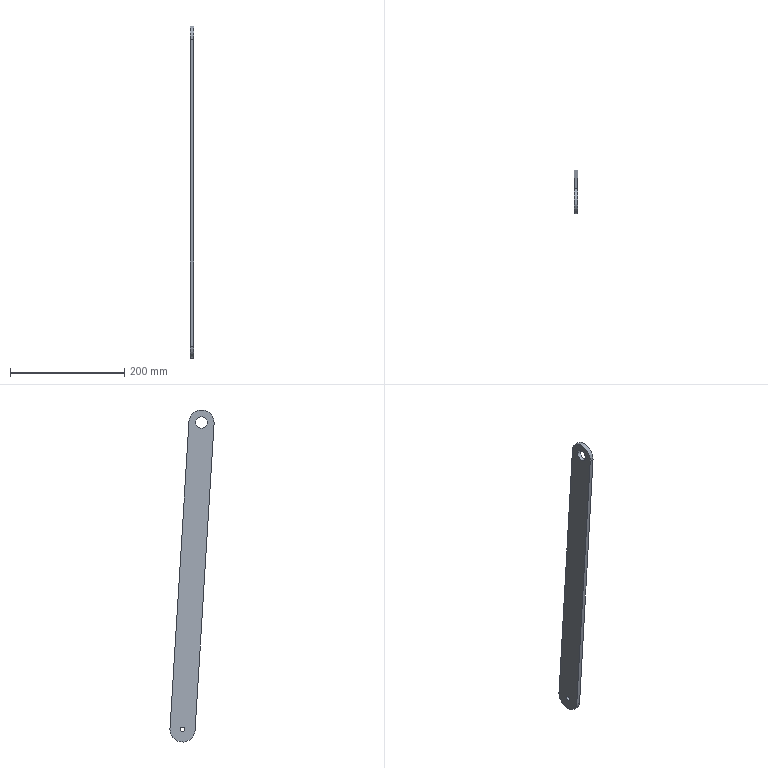Part | SolidWorks | features Extrusion 1 | 1 solid | 11 faces | box 7 x 77.287 x 581.266 mm | volume 173888 mm3 | cylinder 7 | plane 4 | commonest cylinder face diameters 44 x3 8 x2 20 x2
STEP:
#1=CARTESIAN_POINT('',(790.598,-43.287,187.266));
#2=VERTEX_POINT('',#1);
#3=CARTESIAN_POINT('',(790.598,-23.287,187.266));
#4=VERTEX_POINT('',#3);
#5=CARTESIAN_POINT('',(790.598,-33.287,187.266));
#6=DIRECTION('',(1.,0.,0.));
#7=DIRECTION('',(0.,1.,0.));
#8=AXIS2_PLACEMENT_3D('',#5,#6,#7);
#9=CIRCLE('',#8,10.);
#10=EDGE_CURVE('',#2,#4,#9,.T.);
#11=ORIENTED_EDGE('',*,*,#10,.F.);
#12=CARTESIAN_POINT('',(797.598,-43.287,187.266));
#13=VERTEX_POINT('',#12);
#14=CARTESIAN_POINT('',(790.598,-43.287,187.266));
#15=DIRECTION('',(1.,0.,0.));
#16=VECTOR('',#15,1000.);
#17=LINE('',#14,#16);
#18=EDGE_CURVE('',#2,#13,#17,.T.);
#19=ORIENTED_EDGE('',*,*,#18,.T.);
#20=CARTESIAN_POINT('',(797.598,-23.287,187.266));
#21=VERTEX_POINT('',#20);
#22=CARTESIAN_POINT('',(797.598,-33.287,187.266));
#23=DIRECTION('',(1.,0.,0.));
#24=DIRECTION('',(0.,1.,0.));
#25=AXIS2_PLACEMENT_3D('',#22,#23,#24);
#26=CIRCLE('',#25,10.);
#27=EDGE_CURVE('',#13,#21,#26,.T.);
#28=ORIENTED_EDGE('',*,*,#27,.T.);
#29=CARTESIAN_POINT('',(790.598,-23.287,187.266));
#30=DIRECTION('',(1.,0.,0.));
#31=VECTOR('',#30,1000.);
#32=LINE('',#29,#31);
#33=EDGE_CURVE('',#4,#21,#32,.T.);
#34=ORIENTED_EDGE('',*,*,#33,.F.);
#35=EDGE_LOOP('',(#11,#19,#28,#34));
#36=FACE_OUTER_BOUND('',#35,.T.);
#37=CARTESIAN_POINT('',(790.598,-33.287,187.266));
#38=DIRECTION('',(1.,0.,0.));
#39=DIRECTION('',(0.,1.,0.));
#40=AXIS2_PLACEMENT_3D('',#37,#38,#39);
#41=CYLINDRICAL_SURFACE('',#40,10.);
#42=ADVANCED_FACE('',(#36),#41,.F.);
#43=CARTESIAN_POINT('',(790.598,-4.,-350.));
#44=VERTEX_POINT('',#43);
#45=CARTESIAN_POINT('',(790.598,4.,-350.));
#46=VERTEX_POINT('',#45);
#47=CARTESIAN_POINT('',(790.598,0.,-350.));
#48=DIRECTION('',(1.,0.,0.));
#49=DIRECTION('',(0.,1.,0.));
#50=AXIS2_PLACEMENT_3D('',#47,#48,#49);
#51=CIRCLE('',#50,4.);
#52=EDGE_CURVE('',#44,#46,#51,.T.);
#53=ORIENTED_EDGE('',*,*,#52,.F.);
#54=CARTESIAN_POINT('',(797.598,-4.,-350.));
#55=VERTEX_POINT('',#54);
#56=CARTESIAN_POINT('',(790.598,-4.,-350.));
#57=DIRECTION('',(1.,0.,0.));
#58=VECTOR('',#57,1000.);
#59=LINE('',#56,#58);
#60=EDGE_CURVE('',#44,#55,#59,.T.);
#61=ORIENTED_EDGE('',*,*,#60,.T.);
#62=CARTESIAN_POINT('',(797.598,4.,-350.));
#63=VERTEX_POINT('',#62);
#64=CARTESIAN_POINT('',(797.598,0.,-350.));
#65=DIRECTION('',(1.,0.,0.));
#66=DIRECTION('',(0.,1.,0.));
#67=AXIS2_PLACEMENT_3D('',#64,#65,#66);
#68=CIRCLE('',#67,4.);
#69=EDGE_CURVE('',#55,#63,#68,.T.);
#70=ORIENTED_EDGE('',*,*,#69,.T.);
#71=CARTESIAN_POINT('',(790.598,4.,-350.));
#72=DIRECTION('',(1.,0.,0.));
#73=VECTOR('',#72,1000.);
#74=LINE('',#71,#73);
#75=EDGE_CURVE('',#46,#63,#74,.T.);
#76=ORIENTED_EDGE('',*,*,#75,.F.);
#77=EDGE_LOOP('',(#53,#61,#70,#76));
#78=FACE_OUTER_BOUND('',#77,.T.);
#79=CARTESIAN_POINT('',(790.598,0.,-350.));
#80=DIRECTION('',(1.,0.,0.));
#81=DIRECTION('',(0.,1.,0.));
#82=AXIS2_PLACEMENT_3D('',#79,#80,#81);
#83=CYLINDRICAL_SURFACE('',#82,4.);
#84=ADVANCED_FACE('',(#78),#83,.F.);
#85=CARTESIAN_POINT('',(790.598,-21.958,-351.36));
#86=VERTEX_POINT('',#85);
#87=CARTESIAN_POINT('',(790.598,22.,-350.));
#88=VERTEX_POINT('',#87);
#89=CARTESIAN_POINT('',(790.598,0.,-350.));
#90=DIRECTION('',(1.,0.,0.));
#91=DIRECTION('',(0.,1.,0.));
#92=AXIS2_PLACEMENT_3D('',#89,#90,#91);
#93=CIRCLE('',#92,22.);
#94=EDGE_CURVE('',#86,#88,#93,.T.);
#95=ORIENTED_EDGE('',*,*,#94,.T.);
#96=CARTESIAN_POINT('',(797.598,22.,-350.));
#97=VERTEX_POINT('',#96);
#98=CARTESIAN_POINT('',(790.598,22.,-350.));
#99=DIRECTION('',(1.,0.,0.));
#100=VECTOR('',#99,1000.);
#101=LINE('',#98,#100);
#102=EDGE_CURVE('',#88,#97,#101,.T.);
#103=ORIENTED_EDGE('',*,*,#102,.T.);
#104=CARTESIAN_POINT('',(797.598,-21.958,-351.36));
#105=VERTEX_POINT('',#104);
#106=CARTESIAN_POINT('',(797.598,0.,-350.));
#107=DIRECTION('',(1.,0.,0.));
#108=DIRECTION('',(0.,1.,0.));
#109=AXIS2_PLACEMENT_3D('',#106,#107,#108);
#110=CIRCLE('',#109,22.);
#111=EDGE_CURVE('',#105,#97,#110,.T.);
#112=ORIENTED_EDGE('',*,*,#111,.F.);
#113=CARTESIAN_POINT('',(790.598,-21.958,-351.36));
#114=DIRECTION('',(1.,0.,0.));
#115=VECTOR('',#114,1000.);
#116=LINE('',#113,#115);
#117=EDGE_CURVE('',#86,#105,#116,.T.);
#118=ORIENTED_EDGE('',*,*,#117,.F.);
#119=EDGE_LOOP('',(#95,#103,#112,#118));
#120=FACE_OUTER_BOUND('',#119,.T.);
#121=CARTESIAN_POINT('',(790.598,0.,-350.));
#122=DIRECTION('',(1.,0.,0.));
#123=DIRECTION('',(0.,1.,0.));
#124=AXIS2_PLACEMENT_3D('',#121,#122,#123);
#125=CYLINDRICAL_SURFACE('',#124,22.);
#126=ADVANCED_FACE('',(#120),#125,.T.);
#127=CARTESIAN_POINT('',(797.598,-11.33,188.626));
#128=VERTEX_POINT('',#127);
#129=CARTESIAN_POINT('',(797.598,-55.245,185.905));
#130=VERTEX_POINT('',#129);
#131=CARTESIAN_POINT('',(797.598,-33.287,187.266));
#132=DIRECTION('',(1.,0.,0.));
#133=DIRECTION('',(0.,1.,0.));
#134=AXIS2_PLACEMENT_3D('',#131,#132,#133);
#135=CIRCLE('',#134,22.);
#136=EDGE_CURVE('',#128,#130,#135,.T.);
#137=ORIENTED_EDGE('',*,*,#136,.F.);
#138=CARTESIAN_POINT('',(790.598,-11.33,188.626));
#139=VERTEX_POINT('',#138);
#140=CARTESIAN_POINT('',(790.598,-11.33,188.626));
#141=DIRECTION('',(1.,0.,0.));
#142=VECTOR('',#141,1000.);
#143=LINE('',#140,#142);
#144=EDGE_CURVE('',#139,#128,#143,.T.);
#145=ORIENTED_EDGE('',*,*,#144,.F.);
#146=CARTESIAN_POINT('',(790.598,-55.245,185.905));
#147=VERTEX_POINT('',#146);
#148=CARTESIAN_POINT('',(790.598,-33.287,187.266));
#149=DIRECTION('',(1.,0.,0.));
#150=DIRECTION('',(0.,1.,0.));
#151=AXIS2_PLACEMENT_3D('',#148,#149,#150);
#152=CIRCLE('',#151,22.);
#153=EDGE_CURVE('',#139,#147,#152,.T.);
#154=ORIENTED_EDGE('',*,*,#153,.T.);
#155=CARTESIAN_POINT('',(790.598,-55.245,185.905));
#156=DIRECTION('',(1.,0.,0.));
#157=VECTOR('',#156,1000.);
#158=LINE('',#155,#157);
#159=EDGE_CURVE('',#147,#130,#158,.T.);
#160=ORIENTED_EDGE('',*,*,#159,.T.);
#161=EDGE_LOOP('',(#137,#145,#154,#160));
#162=FACE_OUTER_BOUND('',#161,.T.);
#163=CARTESIAN_POINT('',(790.598,-33.287,187.266));
#164=DIRECTION('',(1.,0.,0.));
#165=DIRECTION('',(0.,1.,0.));
#166=AXIS2_PLACEMENT_3D('',#163,#164,#165);
#167=CYLINDRICAL_SURFACE('',#166,22.);
#168=ADVANCED_FACE('',(#162),#167,.T.);
#169=CARTESIAN_POINT('',(797.598,21.958,-348.64));
#170=VERTEX_POINT('',#169);
#171=CARTESIAN_POINT('',(797.598,-11.33,188.626));
#172=DIRECTION('',(0.,-0.06184,0.9981));
#173=VECTOR('',#172,1000.);
#174=LINE('',#171,#173);
#175=EDGE_CURVE('',#170,#128,#174,.T.);
#176=ORIENTED_EDGE('',*,*,#175,.F.);
#177=CARTESIAN_POINT('',(790.598,21.958,-348.64));
#178=VERTEX_POINT('',#177);
#179=CARTESIAN_POINT('',(790.598,21.958,-348.64));
#180=DIRECTION('',(1.,0.,0.));
#181=VECTOR('',#180,1000.);
#182=LINE('',#179,#181);
#183=EDGE_CURVE('',#178,#170,#182,.T.);
#184=ORIENTED_EDGE('',*,*,#183,.F.);
#185=CARTESIAN_POINT('',(790.598,-11.33,188.626));
#186=DIRECTION('',(0.,-0.06184,0.9981));
#187=VECTOR('',#186,1000.);
#188=LINE('',#185,#187);
#189=EDGE_CURVE('',#178,#139,#188,.T.);
#190=ORIENTED_EDGE('',*,*,#189,.T.);
#191=ORIENTED_EDGE('',*,*,#144,.T.);
#192=EDGE_LOOP('',(#176,#184,#190,#191));
#193=FACE_OUTER_BOUND('',#192,.T.);
#194=CARTESIAN_POINT('',(790.598,-11.33,188.626));
#195=DIRECTION('',(0.,0.9981,0.06184));
#196=DIRECTION('',(0.,-0.06184,0.9981));
#197=AXIS2_PLACEMENT_3D('',#194,#195,#196);
#198=PLANE('',#197);
#199=ADVANCED_FACE('',(#193),#198,.T.);
#200=ORIENTED_EDGE('',*,*,#102,.F.);
#201=CARTESIAN_POINT('',(790.598,0.,-350.));
#202=DIRECTION('',(1.,0.,0.));
#203=DIRECTION('',(0.,1.,0.));
#204=AXIS2_PLACEMENT_3D('',#201,#202,#203);
#205=CIRCLE('',#204,22.);
#206=EDGE_CURVE('',#88,#178,#205,.T.);
#207=ORIENTED_EDGE('',*,*,#206,.T.);
#208=ORIENTED_EDGE('',*,*,#183,.T.);
#209=CARTESIAN_POINT('',(797.598,0.,-350.));
#210=DIRECTION('',(1.,0.,0.));
#211=DIRECTION('',(0.,1.,0.));
#212=AXIS2_PLACEMENT_3D('',#209,#210,#211);
#213=CIRCLE('',#212,22.);
#214=EDGE_CURVE('',#97,#170,#213,.T.);
#215=ORIENTED_EDGE('',*,*,#214,.F.);
#216=EDGE_LOOP('',(#200,#207,#208,#215));
#217=FACE_OUTER_BOUND('',#216,.T.);
#218=CARTESIAN_POINT('',(790.598,0.,-350.));
#219=DIRECTION('',(1.,0.,0.));
#220=DIRECTION('',(0.,1.,0.));
#221=AXIS2_PLACEMENT_3D('',#218,#219,#220);
#222=CYLINDRICAL_SURFACE('',#221,22.);
#223=ADVANCED_FACE('',(#217),#222,.T.);
#224=CARTESIAN_POINT('',(797.598,-55.245,185.905));
#225=DIRECTION('',(0.,0.06184,-0.9981));
#226=VECTOR('',#225,1000.);
#227=LINE('',#224,#226);
#228=EDGE_CURVE('',#130,#105,#227,.T.);
#229=ORIENTED_EDGE('',*,*,#228,.F.);
#230=ORIENTED_EDGE('',*,*,#159,.F.);
#231=CARTESIAN_POINT('',(790.598,-55.245,185.905));
#232=DIRECTION('',(0.,0.06184,-0.9981));
#233=VECTOR('',#232,1000.);
#234=LINE('',#231,#233);
#235=EDGE_CURVE('',#147,#86,#234,.T.);
#236=ORIENTED_EDGE('',*,*,#235,.T.);
#237=ORIENTED_EDGE('',*,*,#117,.T.);
#238=EDGE_LOOP('',(#229,#230,#236,#237));
#239=FACE_OUTER_BOUND('',#238,.T.);
#240=CARTESIAN_POINT('',(790.598,-55.245,185.905));
#241=DIRECTION('',(0.,-0.9981,-0.06184));
#242=DIRECTION('',(0.,0.06184,-0.9981));
#243=AXIS2_PLACEMENT_3D('',#240,#241,#242);
#244=PLANE('',#243);
#245=ADVANCED_FACE('',(#239),#244,.T.);
#246=CARTESIAN_POINT('',(790.598,-33.287,187.266));
#247=DIRECTION('',(1.,0.,0.));
#248=DIRECTION('',(0.,1.,0.));
#249=AXIS2_PLACEMENT_3D('',#246,#247,#248);
#250=CIRCLE('',#249,10.);
#251=EDGE_CURVE('',#4,#2,#250,.T.);
#252=ORIENTED_EDGE('',*,*,#251,.T.);
#253=ORIENTED_EDGE('',*,*,#10,.T.);
#254=EDGE_LOOP('',(#252,#253));
#255=FACE_BOUND('',#254,.T.);
#256=CARTESIAN_POINT('',(790.598,0.,-350.));
#257=DIRECTION('',(1.,0.,0.));
#258=DIRECTION('',(0.,1.,0.));
#259=AXIS2_PLACEMENT_3D('',#256,#257,#258);
#260=CIRCLE('',#259,4.);
#261=EDGE_CURVE('',#46,#44,#260,.T.);
#262=ORIENTED_EDGE('',*,*,#261,.T.);
#263=ORIENTED_EDGE('',*,*,#52,.T.);
#264=EDGE_LOOP('',(#262,#263));
#265=FACE_BOUND('',#264,.T.);
#266=ORIENTED_EDGE('',*,*,#153,.F.);
#267=ORIENTED_EDGE('',*,*,#189,.F.);
#268=ORIENTED_EDGE('',*,*,#206,.F.);
#269=ORIENTED_EDGE('',*,*,#94,.F.);
#270=ORIENTED_EDGE('',*,*,#235,.F.);
#271=EDGE_LOOP('',(#266,#267,#268,#269,#270));
#272=FACE_OUTER_BOUND('',#271,.T.);
#273=CARTESIAN_POINT('',(790.598,-33.287,187.266));
#274=DIRECTION('',(1.,0.,0.));
#275=DIRECTION('',(0.,1.,0.));
#276=AXIS2_PLACEMENT_3D('',#273,#274,#275);
#277=PLANE('',#276);
#278=ADVANCED_FACE('',(#255,#265,#272),#277,.F.);
#279=CARTESIAN_POINT('',(797.598,-33.287,187.266));
#280=DIRECTION('',(1.,0.,0.));
#281=DIRECTION('',(0.,1.,0.));
#282=AXIS2_PLACEMENT_3D('',#279,#280,#281);
#283=CIRCLE('',#282,10.);
#284=EDGE_CURVE('',#21,#13,#283,.T.);
#285=ORIENTED_EDGE('',*,*,#284,.F.);
#286=ORIENTED_EDGE('',*,*,#27,.F.);
#287=EDGE_LOOP('',(#285,#286));
#288=FACE_BOUND('',#287,.T.);
#289=CARTESIAN_POINT('',(797.598,0.,-350.));
#290=DIRECTION('',(1.,0.,0.));
#291=DIRECTION('',(0.,1.,0.));
#292=AXIS2_PLACEMENT_3D('',#289,#290,#291);
#293=CIRCLE('',#292,4.);
#294=EDGE_CURVE('',#63,#55,#293,.T.);
#295=ORIENTED_EDGE('',*,*,#294,.F.);
#296=ORIENTED_EDGE('',*,*,#69,.F.);
#297=EDGE_LOOP('',(#295,#296));
#298=FACE_BOUND('',#297,.T.);
#299=ORIENTED_EDGE('',*,*,#136,.T.);
#300=ORIENTED_EDGE('',*,*,#228,.T.);
#301=ORIENTED_EDGE('',*,*,#111,.T.);
#302=ORIENTED_EDGE('',*,*,#214,.T.);
#303=ORIENTED_EDGE('',*,*,#175,.T.);
#304=EDGE_LOOP('',(#299,#300,#301,#302,#303));
#305=FACE_OUTER_BOUND('',#304,.T.);
#306=CARTESIAN_POINT('',(797.598,-33.287,187.266));
#307=DIRECTION('',(1.,0.,0.));
#308=DIRECTION('',(0.,1.,0.));
#309=AXIS2_PLACEMENT_3D('',#306,#307,#308);
#310=PLANE('',#309);
#311=ADVANCED_FACE('',(#288,#298,#305),#310,.T.);
#312=ORIENTED_EDGE('',*,*,#60,.F.);
#313=ORIENTED_EDGE('',*,*,#261,.F.);
#314=ORIENTED_EDGE('',*,*,#75,.T.);
#315=ORIENTED_EDGE('',*,*,#294,.T.);
#316=EDGE_LOOP('',(#312,#313,#314,#315));
#317=FACE_OUTER_BOUND('',#316,.T.);
#318=CARTESIAN_POINT('',(790.598,0.,-350.));
#319=DIRECTION('',(1.,0.,0.));
#320=DIRECTION('',(0.,1.,0.));
#321=AXIS2_PLACEMENT_3D('',#318,#319,#320);
#322=CYLINDRICAL_SURFACE('',#321,4.);
#323=ADVANCED_FACE('',(#317),#322,.F.);
#324=ORIENTED_EDGE('',*,*,#18,.F.);
#325=ORIENTED_EDGE('',*,*,#251,.F.);
#326=ORIENTED_EDGE('',*,*,#33,.T.);
#327=ORIENTED_EDGE('',*,*,#284,.T.);
#328=EDGE_LOOP('',(#324,#325,#326,#327));
#329=FACE_OUTER_BOUND('',#328,.T.);
#330=CARTESIAN_POINT('',(790.598,-33.287,187.266));
#331=DIRECTION('',(1.,0.,0.));
#332=DIRECTION('',(0.,1.,0.));
#333=AXIS2_PLACEMENT_3D('',#330,#331,#332);
#334=CYLINDRICAL_SURFACE('',#333,10.);
#335=ADVANCED_FACE('',(#329),#334,.F.);
#336=CLOSED_SHELL('',(#42,#84,#126,#168,#199,#223,#245,#278,#311,#323,#335));
#337=MANIFOLD_SOLID_BREP('',#336);
#338=CARTESIAN_POINT('',(0.,0.,0.));
#339=DIRECTION('',(0.,0.,1.));
#340=DIRECTION('',(1.,0.,0.));
#341=AXIS2_PLACEMENT_3D('',#338,#339,#340);
#342=(LENGTH_UNIT()NAMED_UNIT(*)SI_UNIT(.MILLI.,.METRE.));
#343=UNCERTAINTY_MEASURE_WITH_UNIT(LENGTH_MEASURE(0.00001),#342,'','');
#344=(NAMED_UNIT(*)PLANE_ANGLE_UNIT()SI_UNIT($,.RADIAN.));
#345=(NAMED_UNIT(*)SI_UNIT($,.STERADIAN.)SOLID_ANGLE_UNIT());
#346=(GEOMETRIC_REPRESENTATION_CONTEXT(3)GLOBAL_UNCERTAINTY_ASSIGNED_CONTEXT((#343))GLOBAL_UNIT_ASSIGNED_CONTEXT((#342,#344,#345))REPRESENTATION_CONTEXT('',''));
#347=ADVANCED_BREP_SHAPE_REPRESENTATION('',(#337,#341),#346);